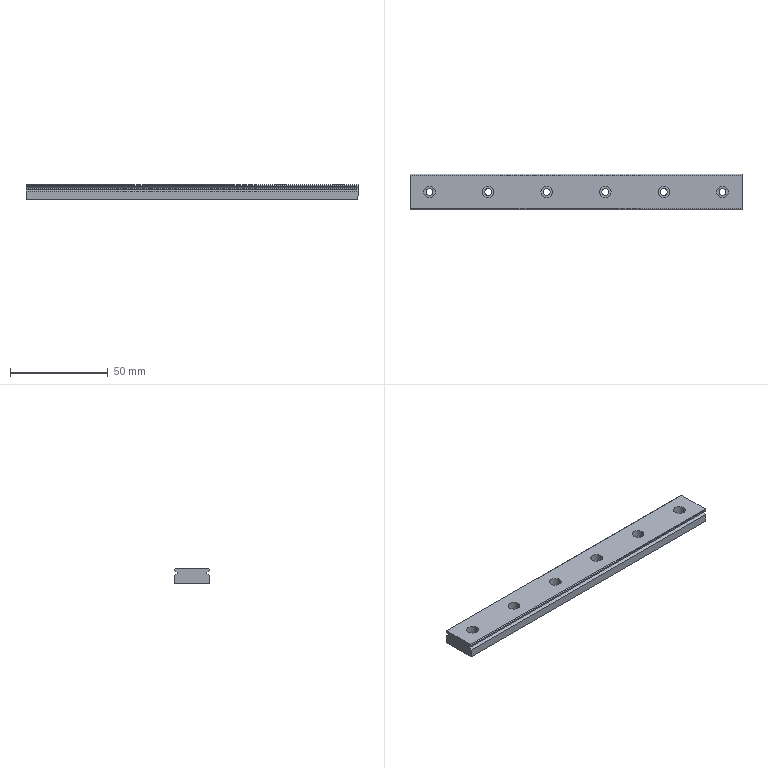Part | SolidWorks | features BaseBody 1 | 1 solid | 46 faces | box 170 x 18 x 7.5 mm | volume 21263 mm3 | cylinder 24 | plane 22 | commonest cylinder face diameters 3.5 x12 6 x12
STEP:
#1=CARTESIAN_POINT('',(-91.75,0.,0.));
#2=VERTEX_POINT('',#1);
#3=CARTESIAN_POINT('',(-88.25,0.,0.));
#4=VERTEX_POINT('',#3);
#5=CARTESIAN_POINT('',(-90.,0.,0.));
#6=DIRECTION('',(0.,0.,1.));
#7=DIRECTION('',(1.,0.,0.));
#8=AXIS2_PLACEMENT_3D('',#5,#6,#7);
#9=CIRCLE('',#8,1.75);
#10=EDGE_CURVE('',#2,#4,#9,.T.);
#11=ORIENTED_EDGE('',*,*,#10,.F.);
#12=CARTESIAN_POINT('',(-91.75,0.,3.));
#13=VERTEX_POINT('',#12);
#14=CARTESIAN_POINT('',(-91.75,0.,-1.163));
#15=DIRECTION('',(0.,0.,1.));
#16=VECTOR('',#15,1000.);
#17=LINE('',#14,#16);
#18=EDGE_CURVE('',#2,#13,#17,.T.);
#19=ORIENTED_EDGE('',*,*,#18,.T.);
#20=CARTESIAN_POINT('',(-88.25,0.,3.));
#21=VERTEX_POINT('',#20);
#22=CARTESIAN_POINT('',(-90.,0.,3.));
#23=DIRECTION('',(0.,0.,-1.));
#24=DIRECTION('',(1.,0.,0.));
#25=AXIS2_PLACEMENT_3D('',#22,#23,#24);
#26=CIRCLE('',#25,1.75);
#27=EDGE_CURVE('',#21,#13,#26,.T.);
#28=ORIENTED_EDGE('',*,*,#27,.F.);
#29=CARTESIAN_POINT('',(-88.25,0.,-1.163));
#30=DIRECTION('',(0.,0.,1.));
#31=VECTOR('',#30,1000.);
#32=LINE('',#29,#31);
#33=EDGE_CURVE('',#4,#21,#32,.T.);
#34=ORIENTED_EDGE('',*,*,#33,.F.);
#35=EDGE_LOOP('',(#11,#19,#28,#34));
#36=FACE_OUTER_BOUND('',#35,.T.);
#37=CARTESIAN_POINT('',(-90.,0.,-1.163));
#38=DIRECTION('',(0.,0.,1.));
#39=DIRECTION('',(1.,0.,0.));
#40=AXIS2_PLACEMENT_3D('',#37,#38,#39);
#41=CYLINDRICAL_SURFACE('',#40,1.75);
#42=ADVANCED_FACE('',(#36),#41,.F.);
#43=CARTESIAN_POINT('',(-61.75,0.,0.));
#44=VERTEX_POINT('',#43);
#45=CARTESIAN_POINT('',(-58.25,0.,0.));
#46=VERTEX_POINT('',#45);
#47=CARTESIAN_POINT('',(-60.,0.,0.));
#48=DIRECTION('',(0.,0.,1.));
#49=DIRECTION('',(1.,0.,0.));
#50=AXIS2_PLACEMENT_3D('',#47,#48,#49);
#51=CIRCLE('',#50,1.75);
#52=EDGE_CURVE('',#44,#46,#51,.T.);
#53=ORIENTED_EDGE('',*,*,#52,.F.);
#54=CARTESIAN_POINT('',(-61.75,0.,3.));
#55=VERTEX_POINT('',#54);
#56=CARTESIAN_POINT('',(-61.75,0.,-1.163));
#57=DIRECTION('',(0.,0.,1.));
#58=VECTOR('',#57,1000.);
#59=LINE('',#56,#58);
#60=EDGE_CURVE('',#44,#55,#59,.T.);
#61=ORIENTED_EDGE('',*,*,#60,.T.);
#62=CARTESIAN_POINT('',(-58.25,0.,3.));
#63=VERTEX_POINT('',#62);
#64=CARTESIAN_POINT('',(-60.,0.,3.));
#65=DIRECTION('',(0.,0.,-1.));
#66=DIRECTION('',(1.,0.,0.));
#67=AXIS2_PLACEMENT_3D('',#64,#65,#66);
#68=CIRCLE('',#67,1.75);
#69=EDGE_CURVE('',#63,#55,#68,.T.);
#70=ORIENTED_EDGE('',*,*,#69,.F.);
#71=CARTESIAN_POINT('',(-58.25,0.,-1.163));
#72=DIRECTION('',(0.,0.,1.));
#73=VECTOR('',#72,1000.);
#74=LINE('',#71,#73);
#75=EDGE_CURVE('',#46,#63,#74,.T.);
#76=ORIENTED_EDGE('',*,*,#75,.F.);
#77=EDGE_LOOP('',(#53,#61,#70,#76));
#78=FACE_OUTER_BOUND('',#77,.T.);
#79=CARTESIAN_POINT('',(-60.,0.,-1.163));
#80=DIRECTION('',(0.,0.,1.));
#81=DIRECTION('',(1.,0.,0.));
#82=AXIS2_PLACEMENT_3D('',#79,#80,#81);
#83=CYLINDRICAL_SURFACE('',#82,1.75);
#84=ADVANCED_FACE('',(#78),#83,.F.);
#85=CARTESIAN_POINT('',(-31.75,0.,0.));
#86=VERTEX_POINT('',#85);
#87=CARTESIAN_POINT('',(-28.25,0.,0.));
#88=VERTEX_POINT('',#87);
#89=CARTESIAN_POINT('',(-30.,0.,0.));
#90=DIRECTION('',(0.,0.,1.));
#91=DIRECTION('',(1.,0.,0.));
#92=AXIS2_PLACEMENT_3D('',#89,#90,#91);
#93=CIRCLE('',#92,1.75);
#94=EDGE_CURVE('',#86,#88,#93,.T.);
#95=ORIENTED_EDGE('',*,*,#94,.F.);
#96=CARTESIAN_POINT('',(-31.75,0.,3.));
#97=VERTEX_POINT('',#96);
#98=CARTESIAN_POINT('',(-31.75,0.,-1.163));
#99=DIRECTION('',(0.,0.,1.));
#100=VECTOR('',#99,1000.);
#101=LINE('',#98,#100);
#102=EDGE_CURVE('',#86,#97,#101,.T.);
#103=ORIENTED_EDGE('',*,*,#102,.T.);
#104=CARTESIAN_POINT('',(-28.25,0.,3.));
#105=VERTEX_POINT('',#104);
#106=CARTESIAN_POINT('',(-30.,0.,3.));
#107=DIRECTION('',(0.,0.,-1.));
#108=DIRECTION('',(1.,0.,0.));
#109=AXIS2_PLACEMENT_3D('',#106,#107,#108);
#110=CIRCLE('',#109,1.75);
#111=EDGE_CURVE('',#105,#97,#110,.T.);
#112=ORIENTED_EDGE('',*,*,#111,.F.);
#113=CARTESIAN_POINT('',(-28.25,0.,-1.163));
#114=DIRECTION('',(0.,0.,1.));
#115=VECTOR('',#114,1000.);
#116=LINE('',#113,#115);
#117=EDGE_CURVE('',#88,#105,#116,.T.);
#118=ORIENTED_EDGE('',*,*,#117,.F.);
#119=EDGE_LOOP('',(#95,#103,#112,#118));
#120=FACE_OUTER_BOUND('',#119,.T.);
#121=CARTESIAN_POINT('',(-30.,0.,-1.163));
#122=DIRECTION('',(0.,0.,1.));
#123=DIRECTION('',(1.,0.,0.));
#124=AXIS2_PLACEMENT_3D('',#121,#122,#123);
#125=CYLINDRICAL_SURFACE('',#124,1.75);
#126=ADVANCED_FACE('',(#120),#125,.F.);
#127=CARTESIAN_POINT('',(58.25,0.,0.));
#128=VERTEX_POINT('',#127);
#129=CARTESIAN_POINT('',(61.75,0.,0.));
#130=VERTEX_POINT('',#129);
#131=CARTESIAN_POINT('',(60.,0.,0.));
#132=DIRECTION('',(0.,0.,1.));
#133=DIRECTION('',(1.,0.,0.));
#134=AXIS2_PLACEMENT_3D('',#131,#132,#133);
#135=CIRCLE('',#134,1.75);
#136=EDGE_CURVE('',#128,#130,#135,.T.);
#137=ORIENTED_EDGE('',*,*,#136,.F.);
#138=CARTESIAN_POINT('',(58.25,0.,3.));
#139=VERTEX_POINT('',#138);
#140=CARTESIAN_POINT('',(58.25,0.,1.5));
#141=DIRECTION('',(0.,0.,1.));
#142=VECTOR('',#141,1000.);
#143=LINE('',#140,#142);
#144=EDGE_CURVE('',#128,#139,#143,.T.);
#145=ORIENTED_EDGE('',*,*,#144,.T.);
#146=CARTESIAN_POINT('',(61.75,0.,3.));
#147=VERTEX_POINT('',#146);
#148=CARTESIAN_POINT('',(60.,0.,3.));
#149=DIRECTION('',(0.,0.,-1.));
#150=DIRECTION('',(1.,0.,0.));
#151=AXIS2_PLACEMENT_3D('',#148,#149,#150);
#152=CIRCLE('',#151,1.75);
#153=EDGE_CURVE('',#147,#139,#152,.T.);
#154=ORIENTED_EDGE('',*,*,#153,.F.);
#155=CARTESIAN_POINT('',(61.75,0.,1.5));
#156=DIRECTION('',(0.,0.,1.));
#157=VECTOR('',#156,1000.);
#158=LINE('',#155,#157);
#159=EDGE_CURVE('',#130,#147,#158,.T.);
#160=ORIENTED_EDGE('',*,*,#159,.F.);
#161=EDGE_LOOP('',(#137,#145,#154,#160));
#162=FACE_OUTER_BOUND('',#161,.T.);
#163=CARTESIAN_POINT('',(60.,0.,1.5));
#164=DIRECTION('',(0.,0.,1.));
#165=DIRECTION('',(1.,0.,0.));
#166=AXIS2_PLACEMENT_3D('',#163,#164,#165);
#167=CYLINDRICAL_SURFACE('',#166,1.75);
#168=ADVANCED_FACE('',(#162),#167,.F.);
#169=CARTESIAN_POINT('',(-1.75,0.,0.));
#170=VERTEX_POINT('',#169);
#171=CARTESIAN_POINT('',(1.75,0.,0.));
#172=VERTEX_POINT('',#171);
#173=CARTESIAN_POINT('',(0.,0.,0.));
#174=DIRECTION('',(0.,0.,1.));
#175=DIRECTION('',(1.,0.,0.));
#176=AXIS2_PLACEMENT_3D('',#173,#174,#175);
#177=CIRCLE('',#176,1.75);
#178=EDGE_CURVE('',#170,#172,#177,.T.);
#179=ORIENTED_EDGE('',*,*,#178,.F.);
#180=CARTESIAN_POINT('',(-1.75,0.,3.));
#181=VERTEX_POINT('',#180);
#182=CARTESIAN_POINT('',(-1.75,0.,1.5));
#183=DIRECTION('',(0.,0.,1.));
#184=VECTOR('',#183,1000.);
#185=LINE('',#182,#184);
#186=EDGE_CURVE('',#170,#181,#185,.T.);
#187=ORIENTED_EDGE('',*,*,#186,.T.);
#188=CARTESIAN_POINT('',(1.75,0.,3.));
#189=VERTEX_POINT('',#188);
#190=CARTESIAN_POINT('',(0.,0.,3.));
#191=DIRECTION('',(0.,0.,-1.));
#192=DIRECTION('',(1.,0.,0.));
#193=AXIS2_PLACEMENT_3D('',#190,#191,#192);
#194=CIRCLE('',#193,1.75);
#195=EDGE_CURVE('',#189,#181,#194,.T.);
#196=ORIENTED_EDGE('',*,*,#195,.F.);
#197=CARTESIAN_POINT('',(1.75,0.,1.5));
#198=DIRECTION('',(0.,0.,1.));
#199=VECTOR('',#198,1000.);
#200=LINE('',#197,#199);
#201=EDGE_CURVE('',#172,#189,#200,.T.);
#202=ORIENTED_EDGE('',*,*,#201,.F.);
#203=EDGE_LOOP('',(#179,#187,#196,#202));
#204=FACE_OUTER_BOUND('',#203,.T.);
#205=CARTESIAN_POINT('',(0.,0.,1.5));
#206=DIRECTION('',(0.,0.,1.));
#207=DIRECTION('',(1.,0.,0.));
#208=AXIS2_PLACEMENT_3D('',#205,#206,#207);
#209=CYLINDRICAL_SURFACE('',#208,1.75);
#210=ADVANCED_FACE('',(#204),#209,.F.);
#211=CARTESIAN_POINT('',(28.25,0.,0.));
#212=VERTEX_POINT('',#211);
#213=CARTESIAN_POINT('',(31.75,0.,0.));
#214=VERTEX_POINT('',#213);
#215=CARTESIAN_POINT('',(30.,0.,0.));
#216=DIRECTION('',(0.,0.,1.));
#217=DIRECTION('',(1.,0.,0.));
#218=AXIS2_PLACEMENT_3D('',#215,#216,#217);
#219=CIRCLE('',#218,1.75);
#220=EDGE_CURVE('',#212,#214,#219,.T.);
#221=ORIENTED_EDGE('',*,*,#220,.F.);
#222=CARTESIAN_POINT('',(28.25,0.,3.));
#223=VERTEX_POINT('',#222);
#224=CARTESIAN_POINT('',(28.25,0.,1.5));
#225=DIRECTION('',(0.,0.,1.));
#226=VECTOR('',#225,1000.);
#227=LINE('',#224,#226);
#228=EDGE_CURVE('',#212,#223,#227,.T.);
#229=ORIENTED_EDGE('',*,*,#228,.T.);
#230=CARTESIAN_POINT('',(31.75,0.,3.));
#231=VERTEX_POINT('',#230);
#232=CARTESIAN_POINT('',(30.,0.,3.));
#233=DIRECTION('',(0.,0.,-1.));
#234=DIRECTION('',(1.,0.,0.));
#235=AXIS2_PLACEMENT_3D('',#232,#233,#234);
#236=CIRCLE('',#235,1.75);
#237=EDGE_CURVE('',#231,#223,#236,.T.);
#238=ORIENTED_EDGE('',*,*,#237,.F.);
#239=CARTESIAN_POINT('',(31.75,0.,1.5));
#240=DIRECTION('',(0.,0.,1.));
#241=VECTOR('',#240,1000.);
#242=LINE('',#239,#241);
#243=EDGE_CURVE('',#214,#231,#242,.T.);
#244=ORIENTED_EDGE('',*,*,#243,.F.);
#245=EDGE_LOOP('',(#221,#229,#238,#244));
#246=FACE_OUTER_BOUND('',#245,.T.);
#247=CARTESIAN_POINT('',(30.,0.,1.5));
#248=DIRECTION('',(0.,0.,1.));
#249=DIRECTION('',(1.,0.,0.));
#250=AXIS2_PLACEMENT_3D('',#247,#248,#249);
#251=CYLINDRICAL_SURFACE('',#250,1.75);
#252=ADVANCED_FACE('',(#246),#251,.F.);
#253=CARTESIAN_POINT('',(-93.,0.,3.));
#254=VERTEX_POINT('',#253);
#255=CARTESIAN_POINT('',(-87.,0.,3.));
#256=VERTEX_POINT('',#255);
#257=CARTESIAN_POINT('',(-90.,0.,3.));
#258=DIRECTION('',(0.,0.,1.));
#259=DIRECTION('',(1.,0.,0.));
#260=AXIS2_PLACEMENT_3D('',#257,#258,#259);
#261=CIRCLE('',#260,3.);
#262=EDGE_CURVE('',#254,#256,#261,.T.);
#263=ORIENTED_EDGE('',*,*,#262,.F.);
#264=CARTESIAN_POINT('',(-93.,0.,7.5));
#265=VERTEX_POINT('',#264);
#266=CARTESIAN_POINT('',(-93.,0.,-1.163));
#267=DIRECTION('',(0.,0.,1.));
#268=VECTOR('',#267,1000.);
#269=LINE('',#266,#268);
#270=EDGE_CURVE('',#254,#265,#269,.T.);
#271=ORIENTED_EDGE('',*,*,#270,.T.);
#272=CARTESIAN_POINT('',(-87.,0.,7.5));
#273=VERTEX_POINT('',#272);
#274=CARTESIAN_POINT('',(-90.,0.,7.5));
#275=DIRECTION('',(0.,0.,-1.));
#276=DIRECTION('',(1.,0.,0.));
#277=AXIS2_PLACEMENT_3D('',#274,#275,#276);
#278=CIRCLE('',#277,3.);
#279=EDGE_CURVE('',#273,#265,#278,.T.);
#280=ORIENTED_EDGE('',*,*,#279,.F.);
#281=CARTESIAN_POINT('',(-87.,0.,-1.163));
#282=DIRECTION('',(0.,0.,1.));
#283=VECTOR('',#282,1000.);
#284=LINE('',#281,#283);
#285=EDGE_CURVE('',#256,#273,#284,.T.);
#286=ORIENTED_EDGE('',*,*,#285,.F.);
#287=EDGE_LOOP('',(#263,#271,#280,#286));
#288=FACE_OUTER_BOUND('',#287,.T.);
#289=CARTESIAN_POINT('',(-90.,0.,-1.163));
#290=DIRECTION('',(0.,0.,1.));
#291=DIRECTION('',(1.,0.,0.));
#292=AXIS2_PLACEMENT_3D('',#289,#290,#291);
#293=CYLINDRICAL_SURFACE('',#292,3.);
#294=ADVANCED_FACE('',(#288),#293,.F.);
#295=CARTESIAN_POINT('',(-63.,0.,3.));
#296=VERTEX_POINT('',#295);
#297=CARTESIAN_POINT('',(-57.,0.,3.));
#298=VERTEX_POINT('',#297);
#299=CARTESIAN_POINT('',(-60.,0.,3.));
#300=DIRECTION('',(0.,0.,1.));
#301=DIRECTION('',(1.,0.,0.));
#302=AXIS2_PLACEMENT_3D('',#299,#300,#301);
#303=CIRCLE('',#302,3.);
#304=EDGE_CURVE('',#296,#298,#303,.T.);
#305=ORIENTED_EDGE('',*,*,#304,.F.);
#306=CARTESIAN_POINT('',(-63.,0.,7.5));
#307=VERTEX_POINT('',#306);
#308=CARTESIAN_POINT('',(-63.,0.,-1.163));
#309=DIRECTION('',(0.,0.,1.));
#310=VECTOR('',#309,1000.);
#311=LINE('',#308,#310);
#312=EDGE_CURVE('',#296,#307,#311,.T.);
#313=ORIENTED_EDGE('',*,*,#312,.T.);
#314=CARTESIAN_POINT('',(-57.,0.,7.5));
#315=VERTEX_POINT('',#314);
#316=CARTESIAN_POINT('',(-60.,0.,7.5));
#317=DIRECTION('',(0.,0.,-1.));
#318=DIRECTION('',(1.,0.,0.));
#319=AXIS2_PLACEMENT_3D('',#316,#317,#318);
#320=CIRCLE('',#319,3.);
#321=EDGE_CURVE('',#315,#307,#320,.T.);
#322=ORIENTED_EDGE('',*,*,#321,.F.);
#323=CARTESIAN_POINT('',(-57.,0.,-1.163));
#324=DIRECTION('',(0.,0.,1.));
#325=VECTOR('',#324,1000.);
#326=LINE('',#323,#325);
#327=EDGE_CURVE('',#298,#315,#326,.T.);
#328=ORIENTED_EDGE('',*,*,#327,.F.);
#329=EDGE_LOOP('',(#305,#313,#322,#328));
#330=FACE_OUTER_BOUND('',#329,.T.);
#331=CARTESIAN_POINT('',(-60.,0.,-1.163));
#332=DIRECTION('',(0.,0.,1.));
#333=DIRECTION('',(1.,0.,0.));
#334=AXIS2_PLACEMENT_3D('',#331,#332,#333);
#335=CYLINDRICAL_SURFACE('',#334,3.);
#336=ADVANCED_FACE('',(#330),#335,.F.);
#337=CARTESIAN_POINT('',(-33.,0.,3.));
#338=VERTEX_POINT('',#337);
#339=CARTESIAN_POINT('',(-27.,0.,3.));
#340=VERTEX_POINT('',#339);
#341=CARTESIAN_POINT('',(-30.,0.,3.));
#342=DIRECTION('',(0.,0.,1.));
#343=DIRECTION('',(1.,0.,0.));
#344=AXIS2_PLACEMENT_3D('',#341,#342,#343);
#345=CIRCLE('',#344,3.);
#346=EDGE_CURVE('',#338,#340,#345,.T.);
#347=ORIENTED_EDGE('',*,*,#346,.F.);
#348=CARTESIAN_POINT('',(-33.,0.,7.5));
#349=VERTEX_POINT('',#348);
#350=CARTESIAN_POINT('',(-33.,0.,-1.163));
#351=DIRECTION('',(0.,0.,1.));
#352=VECTOR('',#351,1000.);
#353=LINE('',#350,#352);
#354=EDGE_CURVE('',#338,#349,#353,.T.);
#355=ORIENTED_EDGE('',*,*,#354,.T.);
#356=CARTESIAN_POINT('',(-27.,0.,7.5));
#357=VERTEX_POINT('',#356);
#358=CARTESIAN_POINT('',(-30.,0.,7.5));
#359=DIRECTION('',(0.,0.,-1.));
#360=DIRECTION('',(1.,0.,0.));
#361=AXIS2_PLACEMENT_3D('',#358,#359,#360);
#362=CIRCLE('',#361,3.);
#363=EDGE_CURVE('',#357,#349,#362,.T.);
#364=ORIENTED_EDGE('',*,*,#363,.F.);
#365=CARTESIAN_POINT('',(-27.,0.,-1.163));
#366=DIRECTION('',(0.,0.,1.));
#367=VECTOR('',#366,1000.);
#368=LINE('',#365,#367);
#369=EDGE_CURVE('',#340,#357,#368,.T.);
#370=ORIENTED_EDGE('',*,*,#369,.F.);
#371=EDGE_LOOP('',(#347,#355,#364,#370));
#372=FACE_OUTER_BOUND('',#371,.T.);
#373=CARTESIAN_POINT('',(-30.,0.,-1.163));
#374=DIRECTION('',(0.,0.,1.));
#375=DIRECTION('',(1.,0.,0.));
#376=AXIS2_PLACEMENT_3D('',#373,#374,#375);
#377=CYLINDRICAL_SURFACE('',#376,3.);
#378=ADVANCED_FACE('',(#372),#377,.F.);
#379=CARTESIAN_POINT('',(63.,0.,7.5));
#380=VERTEX_POINT('',#379);
#381=CARTESIAN_POINT('',(57.,0.,7.5));
#382=VERTEX_POINT('',#381);
#383=CARTESIAN_POINT('',(60.,0.,7.5));
#384=DIRECTION('',(0.,0.,-1.));
#385=DIRECTION('',(-1.,0.,0.));
#386=AXIS2_PLACEMENT_3D('',#383,#384,#385);
#387=CIRCLE('',#386,3.);
#388=EDGE_CURVE('',#380,#382,#387,.T.);
#389=ORIENTED_EDGE('',*,*,#388,.F.);
#390=CARTESIAN_POINT('',(63.,0.,3.));
#391=VERTEX_POINT('',#390);
#392=CARTESIAN_POINT('',(63.,0.,5.25));
#393=DIRECTION('',(0.,0.,-1.));
#394=VECTOR('',#393,1000.);
#395=LINE('',#392,#394);
#396=EDGE_CURVE('',#380,#391,#395,.T.);
#397=ORIENTED_EDGE('',*,*,#396,.T.);
#398=CARTESIAN_POINT('',(57.,0.,3.));
#399=VERTEX_POINT('',#398);
#400=CARTESIAN_POINT('',(60.,0.,3.));
#401=DIRECTION('',(0.,0.,-1.));
#402=DIRECTION('',(-1.,0.,0.));
#403=AXIS2_PLACEMENT_3D('',#400,#401,#402);
#404=CIRCLE('',#403,3.);
#405=EDGE_CURVE('',#391,#399,#404,.T.);
#406=ORIENTED_EDGE('',*,*,#405,.T.);
#407=CARTESIAN_POINT('',(57.,0.,5.25));
#408=DIRECTION('',(0.,0.,-1.));
#409=VECTOR('',#408,1000.);
#410=LINE('',#407,#409);
#411=EDGE_CURVE('',#382,#399,#410,.T.);
#412=ORIENTED_EDGE('',*,*,#411,.F.);
#413=EDGE_LOOP('',(#389,#397,#406,#412));
#414=FACE_OUTER_BOUND('',#413,.T.);
#415=CARTESIAN_POINT('',(60.,0.,5.25));
#416=DIRECTION('',(0.,0.,-1.));
#417=DIRECTION('',(-1.,0.,0.));
#418=AXIS2_PLACEMENT_3D('',#415,#416,#417);
#419=CYLINDRICAL_SURFACE('',#418,3.);
#420=ADVANCED_FACE('',(#414),#419,.F.);
#421=CARTESIAN_POINT('',(3.,0.,7.5));
#422=VERTEX_POINT('',#421);
#423=CARTESIAN_POINT('',(-3.,0.,7.5));
#424=VERTEX_POINT('',#423);
#425=CARTESIAN_POINT('',(0.,0.,7.5));
#426=DIRECTION('',(0.,0.,-1.));
#427=DIRECTION('',(-1.,0.,0.));
#428=AXIS2_PLACEMENT_3D('',#425,#426,#427);
#429=CIRCLE('',#428,3.);
#430=EDGE_CURVE('',#422,#424,#429,.T.);
#431=ORIENTED_EDGE('',*,*,#430,.F.);
#432=CARTESIAN_POINT('',(3.,0.,3.));
#433=VERTEX_POINT('',#432);
#434=CARTESIAN_POINT('',(3.,0.,5.25));
#435=DIRECTION('',(0.,0.,-1.));
#436=VECTOR('',#435,1000.);
#437=LINE('',#434,#436);
#438=EDGE_CURVE('',#422,#433,#437,.T.);
#439=ORIENTED_EDGE('',*,*,#438,.T.);
#440=CARTESIAN_POINT('',(-3.,0.,3.));
#441=VERTEX_POINT('',#440);
#442=CARTESIAN_POINT('',(0.,0.,3.));
#443=DIRECTION('',(0.,0.,-1.));
#444=DIRECTION('',(-1.,0.,0.));
#445=AXIS2_PLACEMENT_3D('',#442,#443,#444);
#446=CIRCLE('',#445,3.);
#447=EDGE_CURVE('',#433,#441,#446,.T.);
#448=ORIENTED_EDGE('',*,*,#447,.T.);
#449=CARTESIAN_POINT('',(-3.,0.,5.25));
#450=DIRECTION('',(0.,0.,-1.));
#451=VECTOR('',#450,1000.);
#452=LINE('',#449,#451);
#453=EDGE_CURVE('',#424,#441,#452,.T.);
#454=ORIENTED_EDGE('',*,*,#453,.F.);
#455=EDGE_LOOP('',(#431,#439,#448,#454));
#456=FACE_OUTER_BOUND('',#455,.T.);
#457=CARTESIAN_POINT('',(0.,0.,5.25));
#458=DIRECTION('',(0.,0.,-1.));
#459=DIRECTION('',(-1.,0.,0.));
#460=AXIS2_PLACEMENT_3D('',#457,#458,#459);
#461=CYLINDRICAL_SURFACE('',#460,3.);
#462=ADVANCED_FACE('',(#456),#461,.F.);
#463=CARTESIAN_POINT('',(33.,0.,7.5));
#464=VERTEX_POINT('',#463);
#465=CARTESIAN_POINT('',(27.,0.,7.5));
#466=VERTEX_POINT('',#465);
#467=CARTESIAN_POINT('',(30.,0.,7.5));
#468=DIRECTION('',(0.,0.,-1.));
#469=DIRECTION('',(-1.,0.,0.));
#470=AXIS2_PLACEMENT_3D('',#467,#468,#469);
#471=CIRCLE('',#470,3.);
#472=EDGE_CURVE('',#464,#466,#471,.T.);
#473=ORIENTED_EDGE('',*,*,#472,.F.);
#474=CARTESIAN_POINT('',(33.,0.,3.));
#475=VERTEX_POINT('',#474);
#476=CARTESIAN_POINT('',(33.,0.,5.25));
#477=DIRECTION('',(0.,0.,-1.));
#478=VECTOR('',#477,1000.);
#479=LINE('',#476,#478);
#480=EDGE_CURVE('',#464,#475,#479,.T.);
#481=ORIENTED_EDGE('',*,*,#480,.T.);
#482=CARTESIAN_POINT('',(27.,0.,3.));
#483=VERTEX_POINT('',#482);
#484=CARTESIAN_POINT('',(30.,0.,3.));
#485=DIRECTION('',(0.,0.,-1.));
#486=DIRECTION('',(-1.,0.,0.));
#487=AXIS2_PLACEMENT_3D('',#484,#485,#486);
#488=CIRCLE('',#487,3.);
#489=EDGE_CURVE('',#475,#483,#488,.T.);
#490=ORIENTED_EDGE('',*,*,#489,.T.);
#491=CARTESIAN_POINT('',(27.,0.,5.25));
#492=DIRECTION('',(0.,0.,-1.));
#493=VECTOR('',#492,1000.);
#494=LINE('',#491,#493);
#495=EDGE_CURVE('',#466,#483,#494,.T.);
#496=ORIENTED_EDGE('',*,*,#495,.F.);
#497=EDGE_LOOP('',(#473,#481,#490,#496));
#498=FACE_OUTER_BOUND('',#497,.T.);
#499=CARTESIAN_POINT('',(30.,0.,5.25));
#500=DIRECTION('',(0.,0.,-1.));
#501=DIRECTION('',(-1.,0.,0.));
#502=AXIS2_PLACEMENT_3D('',#499,#500,#501);
#503=CYLINDRICAL_SURFACE('',#502,3.);
#504=ADVANCED_FACE('',(#498),#503,.F.);
#505=CARTESIAN_POINT('',(-90.,0.,0.));
#506=DIRECTION('',(0.,0.,1.));
#507=DIRECTION('',(1.,0.,0.));
#508=AXIS2_PLACEMENT_3D('',#505,#506,#507);
#509=CIRCLE('',#508,1.75);
#510=EDGE_CURVE('',#4,#2,#509,.T.);
#511=ORIENTED_EDGE('',*,*,#510,.T.);
#512=ORIENTED_EDGE('',*,*,#10,.T.);
#513=EDGE_LOOP('',(#511,#512));
#514=FACE_BOUND('',#513,.T.);
#515=CARTESIAN_POINT('',(-60.,0.,0.));
#516=DIRECTION('',(0.,0.,1.));
#517=DIRECTION('',(1.,0.,0.));
#518=AXIS2_PLACEMENT_3D('',#515,#516,#517);
#519=CIRCLE('',#518,1.75);
#520=EDGE_CURVE('',#46,#44,#519,.T.);
#521=ORIENTED_EDGE('',*,*,#520,.T.);
#522=ORIENTED_EDGE('',*,*,#52,.T.);
#523=EDGE_LOOP('',(#521,#522));
#524=FACE_BOUND('',#523,.T.);
#525=CARTESIAN_POINT('',(-30.,0.,0.));
#526=DIRECTION('',(0.,0.,1.));
#527=DIRECTION('',(1.,0.,0.));
#528=AXIS2_PLACEMENT_3D('',#525,#526,#527);
#529=CIRCLE('',#528,1.75);
#530=EDGE_CURVE('',#88,#86,#529,.T.);
#531=ORIENTED_EDGE('',*,*,#530,.T.);
#532=ORIENTED_EDGE('',*,*,#94,.T.);
#533=EDGE_LOOP('',(#531,#532));
#534=FACE_BOUND('',#533,.T.);
#535=CARTESIAN_POINT('',(60.,0.,0.));
#536=DIRECTION('',(0.,0.,1.));
#537=DIRECTION('',(1.,0.,0.));
#538=AXIS2_PLACEMENT_3D('',#535,#536,#537);
#539=CIRCLE('',#538,1.75);
#540=EDGE_CURVE('',#130,#128,#539,.T.);
#541=ORIENTED_EDGE('',*,*,#540,.T.);
#542=ORIENTED_EDGE('',*,*,#136,.T.);
#543=EDGE_LOOP('',(#541,#542));
#544=FACE_BOUND('',#543,.T.);
#545=CARTESIAN_POINT('',(0.,0.,0.));
#546=DIRECTION('',(0.,0.,1.));
#547=DIRECTION('',(1.,0.,0.));
#548=AXIS2_PLACEMENT_3D('',#545,#546,#547);
#549=CIRCLE('',#548,1.75);
#550=EDGE_CURVE('',#172,#170,#549,.T.);
#551=ORIENTED_EDGE('',*,*,#550,.T.);
#552=ORIENTED_EDGE('',*,*,#178,.T.);
#553=EDGE_LOOP('',(#551,#552));
#554=FACE_BOUND('',#553,.T.);
#555=CARTESIAN_POINT('',(30.,0.,0.));
#556=DIRECTION('',(0.,0.,1.));
#557=DIRECTION('',(1.,0.,0.));
#558=AXIS2_PLACEMENT_3D('',#555,#556,#557);
#559=CIRCLE('',#558,1.75);
#560=EDGE_CURVE('',#214,#212,#559,.T.);
#561=ORIENTED_EDGE('',*,*,#560,.T.);
#562=ORIENTED_EDGE('',*,*,#220,.T.);
#563=EDGE_LOOP('',(#561,#562));
#564=FACE_BOUND('',#563,.T.);
#565=CARTESIAN_POINT('',(-100.,-9.,0.));
#566=VERTEX_POINT('',#565);
#567=CARTESIAN_POINT('',(-100.,9.,0.));
#568=VERTEX_POINT('',#567);
#569=CARTESIAN_POINT('',(-100.,0.,0.));
#570=DIRECTION('',(0.,1.,0.));
#571=VECTOR('',#570,1000.);
#572=LINE('',#569,#571);
#573=EDGE_CURVE('',#566,#568,#572,.T.);
#574=ORIENTED_EDGE('',*,*,#573,.T.);
#575=CARTESIAN_POINT('',(70.,9.,0.));
#576=VERTEX_POINT('',#575);
#577=CARTESIAN_POINT('',(-10.,9.,0.));
#578=DIRECTION('',(1.,0.,0.));
#579=VECTOR('',#578,1000.);
#580=LINE('',#577,#579);
#581=EDGE_CURVE('',#568,#576,#580,.T.);
#582=ORIENTED_EDGE('',*,*,#581,.T.);
#583=CARTESIAN_POINT('',(70.,-9.,0.));
#584=VERTEX_POINT('',#583);
#585=CARTESIAN_POINT('',(70.,0.,0.));
#586=DIRECTION('',(0.,-1.,0.));
#587=VECTOR('',#586,1000.);
#588=LINE('',#585,#587);
#589=EDGE_CURVE('',#576,#584,#588,.T.);
#590=ORIENTED_EDGE('',*,*,#589,.T.);
#591=CARTESIAN_POINT('',(-10.,-9.,0.));
#592=DIRECTION('',(-1.,0.,0.));
#593=VECTOR('',#592,1000.);
#594=LINE('',#591,#593);
#595=EDGE_CURVE('',#584,#566,#594,.T.);
#596=ORIENTED_EDGE('',*,*,#595,.T.);
#597=EDGE_LOOP('',(#574,#582,#590,#596));
#598=FACE_OUTER_BOUND('',#597,.T.);
#599=CARTESIAN_POINT('',(-10.,0.,0.));
#600=DIRECTION('',(0.,0.,-1.));
#601=DIRECTION('',(-1.,0.,0.));
#602=AXIS2_PLACEMENT_3D('',#599,#600,#601);
#603=PLANE('',#602);
#604=ADVANCED_FACE('',(#514,#524,#534,#544,#554,#564,#598),#603,.T.);
#605=ORIENTED_EDGE('',*,*,#18,.F.);
#606=ORIENTED_EDGE('',*,*,#510,.F.);
#607=ORIENTED_EDGE('',*,*,#33,.T.);
#608=CARTESIAN_POINT('',(-90.,0.,3.));
#609=DIRECTION('',(0.,0.,-1.));
#610=DIRECTION('',(1.,0.,0.));
#611=AXIS2_PLACEMENT_3D('',#608,#609,#610);
#612=CIRCLE('',#611,1.75);
#613=EDGE_CURVE('',#13,#21,#612,.T.);
#614=ORIENTED_EDGE('',*,*,#613,.F.);
#615=EDGE_LOOP('',(#605,#606,#607,#614));
#616=FACE_OUTER_BOUND('',#615,.T.);
#617=CARTESIAN_POINT('',(-90.,0.,-1.163));
#618=DIRECTION('',(0.,0.,1.));
#619=DIRECTION('',(1.,0.,0.));
#620=AXIS2_PLACEMENT_3D('',#617,#618,#619);
#621=CYLINDRICAL_SURFACE('',#620,1.75);
#622=ADVANCED_FACE('',(#616),#621,.F.);
#623=ORIENTED_EDGE('',*,*,#60,.F.);
#624=ORIENTED_EDGE('',*,*,#520,.F.);
#625=ORIENTED_EDGE('',*,*,#75,.T.);
#626=CARTESIAN_POINT('',(-60.,0.,3.));
#627=DIRECTION('',(0.,0.,-1.));
#628=DIRECTION('',(1.,0.,0.));
#629=AXIS2_PLACEMENT_3D('',#626,#627,#628);
#630=CIRCLE('',#629,1.75);
#631=EDGE_CURVE('',#55,#63,#630,.T.);
#632=ORIENTED_EDGE('',*,*,#631,.F.);
#633=EDGE_LOOP('',(#623,#624,#625,#632));
#634=FACE_OUTER_BOUND('',#633,.T.);
#635=CARTESIAN_POINT('',(-60.,0.,-1.163));
#636=DIRECTION('',(0.,0.,1.));
#637=DIRECTION('',(1.,0.,0.));
#638=AXIS2_PLACEMENT_3D('',#635,#636,#637);
#639=CYLINDRICAL_SURFACE('',#638,1.75);
#640=ADVANCED_FACE('',(#634),#639,.F.);
#641=ORIENTED_EDGE('',*,*,#102,.F.);
#642=ORIENTED_EDGE('',*,*,#530,.F.);
#643=ORIENTED_EDGE('',*,*,#117,.T.);
#644=CARTESIAN_POINT('',(-30.,0.,3.));
#645=DIRECTION('',(0.,0.,-1.));
#646=DIRECTION('',(1.,0.,0.));
#647=AXIS2_PLACEMENT_3D('',#644,#645,#646);
#648=CIRCLE('',#647,1.75);
#649=EDGE_CURVE('',#97,#105,#648,.T.);
#650=ORIENTED_EDGE('',*,*,#649,.F.);
#651=EDGE_LOOP('',(#641,#642,#643,#650));
#652=FACE_OUTER_BOUND('',#651,.T.);
#653=CARTESIAN_POINT('',(-30.,0.,-1.163));
#654=DIRECTION('',(0.,0.,1.));
#655=DIRECTION('',(1.,0.,0.));
#656=AXIS2_PLACEMENT_3D('',#653,#654,#655);
#657=CYLINDRICAL_SURFACE('',#656,1.75);
#658=ADVANCED_FACE('',(#652),#657,.F.);
#659=ORIENTED_EDGE('',*,*,#144,.F.);
#660=ORIENTED_EDGE('',*,*,#540,.F.);
#661=ORIENTED_EDGE('',*,*,#159,.T.);
#662=CARTESIAN_POINT('',(60.,0.,3.));
#663=DIRECTION('',(0.,0.,-1.));
#664=DIRECTION('',(1.,0.,0.));
#665=AXIS2_PLACEMENT_3D('',#662,#663,#664);
#666=CIRCLE('',#665,1.75);
#667=EDGE_CURVE('',#139,#147,#666,.T.);
#668=ORIENTED_EDGE('',*,*,#667,.F.);
#669=EDGE_LOOP('',(#659,#660,#661,#668));
#670=FACE_OUTER_BOUND('',#669,.T.);
#671=CARTESIAN_POINT('',(60.,0.,1.5));
#672=DIRECTION('',(0.,0.,1.));
#673=DIRECTION('',(1.,0.,0.));
#674=AXIS2_PLACEMENT_3D('',#671,#672,#673);
#675=CYLINDRICAL_SURFACE('',#674,1.75);
#676=ADVANCED_FACE('',(#670),#675,.F.);
#677=ORIENTED_EDGE('',*,*,#186,.F.);
#678=ORIENTED_EDGE('',*,*,#550,.F.);
#679=ORIENTED_EDGE('',*,*,#201,.T.);
#680=CARTESIAN_POINT('',(0.,0.,3.));
#681=DIRECTION('',(0.,0.,-1.));
#682=DIRECTION('',(1.,0.,0.));
#683=AXIS2_PLACEMENT_3D('',#680,#681,#682);
#684=CIRCLE('',#683,1.75);
#685=EDGE_CURVE('',#181,#189,#684,.T.);
#686=ORIENTED_EDGE('',*,*,#685,.F.);
#687=EDGE_LOOP('',(#677,#678,#679,#686));
#688=FACE_OUTER_BOUND('',#687,.T.);
#689=CARTESIAN_POINT('',(0.,0.,1.5));
#690=DIRECTION('',(0.,0.,1.));
#691=DIRECTION('',(1.,0.,0.));
#692=AXIS2_PLACEMENT_3D('',#689,#690,#691);
#693=CYLINDRICAL_SURFACE('',#692,1.75);
#694=ADVANCED_FACE('',(#688),#693,.F.);
#695=ORIENTED_EDGE('',*,*,#228,.F.);
#696=ORIENTED_EDGE('',*,*,#560,.F.);
#697=ORIENTED_EDGE('',*,*,#243,.T.);
#698=CARTESIAN_POINT('',(30.,0.,3.));
#699=DIRECTION('',(0.,0.,-1.));
#700=DIRECTION('',(1.,0.,0.));
#701=AXIS2_PLACEMENT_3D('',#698,#699,#700);
#702=CIRCLE('',#701,1.75);
#703=EDGE_CURVE('',#223,#231,#702,.T.);
#704=ORIENTED_EDGE('',*,*,#703,.F.);
#705=EDGE_LOOP('',(#695,#696,#697,#704));
#706=FACE_OUTER_BOUND('',#705,.T.);
#707=CARTESIAN_POINT('',(30.,0.,1.5));
#708=DIRECTION('',(0.,0.,1.));
#709=DIRECTION('',(1.,0.,0.));
#710=AXIS2_PLACEMENT_3D('',#707,#708,#709);
#711=CYLINDRICAL_SURFACE('',#710,1.75);
#712=ADVANCED_FACE('',(#706),#711,.F.);
#713=CARTESIAN_POINT('',(-100.,9.,4.2));
#714=VERTEX_POINT('',#713);
#715=CARTESIAN_POINT('',(-100.,9.,4.2));
#716=DIRECTION('',(0.,0.,1.));
#717=VECTOR('',#716,1000.);
#718=LINE('',#715,#717);
#719=EDGE_CURVE('',#568,#714,#718,.T.);
#720=ORIENTED_EDGE('',*,*,#719,.T.);
#721=CARTESIAN_POINT('',(70.,9.,4.2));
#722=VERTEX_POINT('',#721);
#723=CARTESIAN_POINT('',(-10.,9.,4.2));
#724=DIRECTION('',(1.,0.,0.));
#725=VECTOR('',#724,1000.);
#726=LINE('',#723,#725);
#727=EDGE_CURVE('',#714,#722,#726,.T.);
#728=ORIENTED_EDGE('',*,*,#727,.T.);
#729=CARTESIAN_POINT('',(70.,9.,4.2));
#730=DIRECTION('',(0.,0.,-1.));
#731=VECTOR('',#730,1000.);
#732=LINE('',#729,#731);
#733=EDGE_CURVE('',#722,#576,#732,.T.);
#734=ORIENTED_EDGE('',*,*,#733,.T.);
#735=ORIENTED_EDGE('',*,*,#581,.F.);
#736=EDGE_LOOP('',(#720,#728,#734,#735));
#737=FACE_OUTER_BOUND('',#736,.T.);
#738=CARTESIAN_POINT('',(-10.,9.,4.2));
#739=DIRECTION('',(0.,1.,0.));
#740=DIRECTION('',(0.,0.,1.));
#741=AXIS2_PLACEMENT_3D('',#738,#739,#740);
#742=PLANE('',#741);
#743=ADVANCED_FACE('',(#737),#742,.T.);
#744=ORIENTED_EDGE('',*,*,#719,.F.);
#745=ORIENTED_EDGE('',*,*,#573,.F.);
#746=CARTESIAN_POINT('',(-100.,-9.,4.2));
#747=VERTEX_POINT('',#746);
#748=CARTESIAN_POINT('',(-100.,-9.,0.));
#749=DIRECTION('',(0.,0.,1.));
#750=VECTOR('',#749,1000.);
#751=LINE('',#748,#750);
#752=EDGE_CURVE('',#566,#747,#751,.T.);
#753=ORIENTED_EDGE('',*,*,#752,.T.);
#754=CARTESIAN_POINT('',(-100.,-7.5,4.95));
#755=VERTEX_POINT('',#754);
#756=CARTESIAN_POINT('',(-100.,-9.,4.2));
#757=DIRECTION('',(0.,-0.8944,-0.4472));
#758=VECTOR('',#757,1000.);
#759=LINE('',#756,#758);
#760=EDGE_CURVE('',#755,#747,#759,.T.);
#761=ORIENTED_EDGE('',*,*,#760,.F.);
#762=CARTESIAN_POINT('',(-100.,-7.5,5.625));
#763=VERTEX_POINT('',#762);
#764=CARTESIAN_POINT('',(-100.,-7.5,4.95));
#765=DIRECTION('',(0.,0.,-1.));
#766=VECTOR('',#765,1000.);
#767=LINE('',#764,#766);
#768=EDGE_CURVE('',#763,#755,#767,.T.);
#769=ORIENTED_EDGE('',*,*,#768,.F.);
#770=CARTESIAN_POINT('',(-100.,-9.,6.375));
#771=VERTEX_POINT('',#770);
#772=CARTESIAN_POINT('',(-100.,-7.5,5.625));
#773=DIRECTION('',(0.,0.8944,-0.4472));
#774=VECTOR('',#773,1000.);
#775=LINE('',#772,#774);
#776=EDGE_CURVE('',#771,#763,#775,.T.);
#777=ORIENTED_EDGE('',*,*,#776,.F.);
#778=CARTESIAN_POINT('',(-100.,-9.,7.125));
#779=VERTEX_POINT('',#778);
#780=CARTESIAN_POINT('',(-100.,-9.,6.375));
#781=DIRECTION('',(0.,0.,-1.));
#782=VECTOR('',#781,1000.);
#783=LINE('',#780,#782);
#784=EDGE_CURVE('',#779,#771,#783,.T.);
#785=ORIENTED_EDGE('',*,*,#784,.F.);
#786=CARTESIAN_POINT('',(-100.,-8.625,7.5));
#787=VERTEX_POINT('',#786);
#788=CARTESIAN_POINT('',(-100.,-9.,7.125));
#789=DIRECTION('',(0.,-0.7071,-0.7071));
#790=VECTOR('',#789,1000.);
#791=LINE('',#788,#790);
#792=EDGE_CURVE('',#787,#779,#791,.T.);
#793=ORIENTED_EDGE('',*,*,#792,.F.);
#794=CARTESIAN_POINT('',(-100.,8.625,7.5));
#795=VERTEX_POINT('',#794);
#796=CARTESIAN_POINT('',(-100.,0.,7.5));
#797=DIRECTION('',(0.,1.,0.));
#798=VECTOR('',#797,1000.);
#799=LINE('',#796,#798);
#800=EDGE_CURVE('',#787,#795,#799,.T.);
#801=ORIENTED_EDGE('',*,*,#800,.T.);
#802=CARTESIAN_POINT('',(-100.,9.,7.125));
#803=VERTEX_POINT('',#802);
#804=CARTESIAN_POINT('',(-100.,8.625,7.5));
#805=DIRECTION('',(0.,-0.7071,0.7071));
#806=VECTOR('',#805,1000.);
#807=LINE('',#804,#806);
#808=EDGE_CURVE('',#803,#795,#807,.T.);
#809=ORIENTED_EDGE('',*,*,#808,.F.);
#810=CARTESIAN_POINT('',(-100.,9.,6.375));
#811=VERTEX_POINT('',#810);
#812=CARTESIAN_POINT('',(-100.,9.,7.125));
#813=DIRECTION('',(0.,0.,1.));
#814=VECTOR('',#813,1000.);
#815=LINE('',#812,#814);
#816=EDGE_CURVE('',#811,#803,#815,.T.);
#817=ORIENTED_EDGE('',*,*,#816,.F.);
#818=CARTESIAN_POINT('',(-100.,7.5,5.625));
#819=VERTEX_POINT('',#818);
#820=CARTESIAN_POINT('',(-100.,9.,6.375));
#821=DIRECTION('',(0.,0.8944,0.4472));
#822=VECTOR('',#821,1000.);
#823=LINE('',#820,#822);
#824=EDGE_CURVE('',#819,#811,#823,.T.);
#825=ORIENTED_EDGE('',*,*,#824,.F.);
#826=CARTESIAN_POINT('',(-100.,7.5,4.95));
#827=VERTEX_POINT('',#826);
#828=CARTESIAN_POINT('',(-100.,7.5,5.625));
#829=DIRECTION('',(0.,0.,1.));
#830=VECTOR('',#829,1000.);
#831=LINE('',#828,#830);
#832=EDGE_CURVE('',#827,#819,#831,.T.);
#833=ORIENTED_EDGE('',*,*,#832,.F.);
#834=CARTESIAN_POINT('',(-100.,7.5,4.95));
#835=DIRECTION('',(0.,0.8944,-0.4472));
#836=VECTOR('',#835,1000.);
#837=LINE('',#834,#836);
#838=EDGE_CURVE('',#827,#714,#837,.T.);
#839=ORIENTED_EDGE('',*,*,#838,.T.);
#840=EDGE_LOOP('',(#744,#745,#753,#761,#769,#777,#785,#793,#801,#809,#817,#825,#833,#839));
#841=FACE_OUTER_BOUND('',#840,.T.);
#842=CARTESIAN_POINT('',(-100.,0.,0.));
#843=DIRECTION('',(-1.,0.,0.));
#844=DIRECTION('',(0.,0.,1.));
#845=AXIS2_PLACEMENT_3D('',#842,#843,#844);
#846=PLANE('',#845);
#847=ADVANCED_FACE('',(#841),#846,.T.);
#848=ORIENTED_EDGE('',*,*,#752,.F.);
#849=ORIENTED_EDGE('',*,*,#595,.F.);
#850=CARTESIAN_POINT('',(70.,-9.,4.2));
#851=VERTEX_POINT('',#850);
#852=CARTESIAN_POINT('',(70.,-9.,0.));
#853=DIRECTION('',(0.,0.,1.));
#854=VECTOR('',#853,1000.);
#855=LINE('',#852,#854);
#856=EDGE_CURVE('',#584,#851,#855,.T.);
#857=ORIENTED_EDGE('',*,*,#856,.T.);
#858=CARTESIAN_POINT('',(-10.,-9.,4.2));
#859=DIRECTION('',(-1.,0.,0.));
#860=VECTOR('',#859,1000.);
#861=LINE('',#858,#860);
#862=EDGE_CURVE('',#851,#747,#861,.T.);
#863=ORIENTED_EDGE('',*,*,#862,.T.);
#864=EDGE_LOOP('',(#848,#849,#857,#863));
#865=FACE_OUTER_BOUND('',#864,.T.);
#866=CARTESIAN_POINT('',(-10.,-9.,0.));
#867=DIRECTION('',(0.,-1.,0.));
#868=DIRECTION('',(0.,0.,-1.));
#869=AXIS2_PLACEMENT_3D('',#866,#867,#868);
#870=PLANE('',#869);
#871=ADVANCED_FACE('',(#865),#870,.T.);
#872=CARTESIAN_POINT('',(70.,7.5,4.95));
#873=VERTEX_POINT('',#872);
#874=CARTESIAN_POINT('',(70.,7.5,4.95));
#875=DIRECTION('',(0.,0.8944,-0.4472));
#876=VECTOR('',#875,1000.);
#877=LINE('',#874,#876);
#878=EDGE_CURVE('',#873,#722,#877,.T.);
#879=ORIENTED_EDGE('',*,*,#878,.F.);
#880=CARTESIAN_POINT('',(70.,7.5,5.625));
#881=VERTEX_POINT('',#880);
#882=CARTESIAN_POINT('',(70.,7.5,5.625));
#883=DIRECTION('',(0.,0.,-1.));
#884=VECTOR('',#883,1000.);
#885=LINE('',#882,#884);
#886=EDGE_CURVE('',#881,#873,#885,.T.);
#887=ORIENTED_EDGE('',*,*,#886,.F.);
#888=CARTESIAN_POINT('',(70.,9.,6.375));
#889=VERTEX_POINT('',#888);
#890=CARTESIAN_POINT('',(70.,9.,6.375));
#891=DIRECTION('',(0.,-0.8944,-0.4472));
#892=VECTOR('',#891,1000.);
#893=LINE('',#890,#892);
#894=EDGE_CURVE('',#889,#881,#893,.T.);
#895=ORIENTED_EDGE('',*,*,#894,.F.);
#896=CARTESIAN_POINT('',(70.,9.,7.125));
#897=VERTEX_POINT('',#896);
#898=CARTESIAN_POINT('',(70.,9.,7.125));
#899=DIRECTION('',(0.,0.,-1.));
#900=VECTOR('',#899,1000.);
#901=LINE('',#898,#900);
#902=EDGE_CURVE('',#897,#889,#901,.T.);
#903=ORIENTED_EDGE('',*,*,#902,.F.);
#904=CARTESIAN_POINT('',(70.,8.625,7.5));
#905=VERTEX_POINT('',#904);
#906=CARTESIAN_POINT('',(70.,8.625,7.5));
#907=DIRECTION('',(0.,0.7071,-0.7071));
#908=VECTOR('',#907,1000.);
#909=LINE('',#906,#908);
#910=EDGE_CURVE('',#905,#897,#909,.T.);
#911=ORIENTED_EDGE('',*,*,#910,.F.);
#912=CARTESIAN_POINT('',(70.,-8.625,7.5));
#913=VERTEX_POINT('',#912);
#914=CARTESIAN_POINT('',(70.,0.,7.5));
#915=DIRECTION('',(0.,1.,0.));
#916=VECTOR('',#915,1000.);
#917=LINE('',#914,#916);
#918=EDGE_CURVE('',#913,#905,#917,.T.);
#919=ORIENTED_EDGE('',*,*,#918,.F.);
#920=CARTESIAN_POINT('',(70.,-9.,7.125));
#921=VERTEX_POINT('',#920);
#922=CARTESIAN_POINT('',(70.,-9.,7.125));
#923=DIRECTION('',(0.,0.7071,0.7071));
#924=VECTOR('',#923,1000.);
#925=LINE('',#922,#924);
#926=EDGE_CURVE('',#921,#913,#925,.T.);
#927=ORIENTED_EDGE('',*,*,#926,.F.);
#928=CARTESIAN_POINT('',(70.,-9.,6.375));
#929=VERTEX_POINT('',#928);
#930=CARTESIAN_POINT('',(70.,-9.,6.375));
#931=DIRECTION('',(0.,0.,1.));
#932=VECTOR('',#931,1000.);
#933=LINE('',#930,#932);
#934=EDGE_CURVE('',#929,#921,#933,.T.);
#935=ORIENTED_EDGE('',*,*,#934,.F.);
#936=CARTESIAN_POINT('',(70.,-7.5,5.625));
#937=VERTEX_POINT('',#936);
#938=CARTESIAN_POINT('',(70.,-7.5,5.625));
#939=DIRECTION('',(0.,-0.8944,0.4472));
#940=VECTOR('',#939,1000.);
#941=LINE('',#938,#940);
#942=EDGE_CURVE('',#937,#929,#941,.T.);
#943=ORIENTED_EDGE('',*,*,#942,.F.);
#944=CARTESIAN_POINT('',(70.,-7.5,4.95));
#945=VERTEX_POINT('',#944);
#946=CARTESIAN_POINT('',(70.,-7.5,4.95));
#947=DIRECTION('',(0.,0.,1.));
#948=VECTOR('',#947,1000.);
#949=LINE('',#946,#948);
#950=EDGE_CURVE('',#945,#937,#949,.T.);
#951=ORIENTED_EDGE('',*,*,#950,.F.);
#952=CARTESIAN_POINT('',(70.,-9.,4.2));
#953=DIRECTION('',(0.,0.8944,0.4472));
#954=VECTOR('',#953,1000.);
#955=LINE('',#952,#954);
#956=EDGE_CURVE('',#851,#945,#955,.T.);
#957=ORIENTED_EDGE('',*,*,#956,.F.);
#958=ORIENTED_EDGE('',*,*,#856,.F.);
#959=ORIENTED_EDGE('',*,*,#589,.F.);
#960=ORIENTED_EDGE('',*,*,#733,.F.);
#961=EDGE_LOOP('',(#879,#887,#895,#903,#911,#919,#927,#935,#943,#951,#957,#958,#959,#960));
#962=FACE_OUTER_BOUND('',#961,.T.);
#963=CARTESIAN_POINT('',(70.,0.,3.824));
#964=DIRECTION('',(-1.,0.,0.));
#965=DIRECTION('',(0.,0.,1.));
#966=AXIS2_PLACEMENT_3D('',#963,#964,#965);
#967=PLANE('',#966);
#968=ADVANCED_FACE('',(#962),#967,.F.);
#969=ORIENTED_EDGE('',*,*,#27,.T.);
#970=ORIENTED_EDGE('',*,*,#613,.T.);
#971=EDGE_LOOP('',(#969,#970));
#972=FACE_BOUND('',#971,.T.);
#973=CARTESIAN_POINT('',(-90.,0.,3.));
#974=DIRECTION('',(0.,0.,1.));
#975=DIRECTION('',(1.,0.,0.));
#976=AXIS2_PLACEMENT_3D('',#973,#974,#975);
#977=CIRCLE('',#976,3.);
#978=EDGE_CURVE('',#256,#254,#977,.T.);
#979=ORIENTED_EDGE('',*,*,#978,.T.);
#980=ORIENTED_EDGE('',*,*,#262,.T.);
#981=EDGE_LOOP('',(#979,#980));
#982=FACE_OUTER_BOUND('',#981,.T.);
#983=CARTESIAN_POINT('',(-90.,0.,3.));
#984=DIRECTION('',(0.,0.,1.));
#985=DIRECTION('',(1.,0.,0.));
#986=AXIS2_PLACEMENT_3D('',#983,#984,#985);
#987=PLANE('',#986);
#988=ADVANCED_FACE('',(#972,#982),#987,.T.);
#989=ORIENTED_EDGE('',*,*,#69,.T.);
#990=ORIENTED_EDGE('',*,*,#631,.T.);
#991=EDGE_LOOP('',(#989,#990));
#992=FACE_BOUND('',#991,.T.);
#993=CARTESIAN_POINT('',(-60.,0.,3.));
#994=DIRECTION('',(0.,0.,1.));
#995=DIRECTION('',(1.,0.,0.));
#996=AXIS2_PLACEMENT_3D('',#993,#994,#995);
#997=CIRCLE('',#996,3.);
#998=EDGE_CURVE('',#298,#296,#997,.T.);
#999=ORIENTED_EDGE('',*,*,#998,.T.);
#1000=ORIENTED_EDGE('',*,*,#304,.T.);
#1001=EDGE_LOOP('',(#999,#1000));
#1002=FACE_OUTER_BOUND('',#1001,.T.);
#1003=CARTESIAN_POINT('',(-60.,0.,3.));
#1004=DIRECTION('',(0.,0.,1.));
#1005=DIRECTION('',(1.,0.,0.));
#1006=AXIS2_PLACEMENT_3D('',#1003,#1004,#1005);
#1007=PLANE('',#1006);
#1008=ADVANCED_FACE('',(#992,#1002),#1007,.T.);
#1009=ORIENTED_EDGE('',*,*,#111,.T.);
#1010=ORIENTED_EDGE('',*,*,#649,.T.);
#1011=EDGE_LOOP('',(#1009,#1010));
#1012=FACE_BOUND('',#1011,.T.);
#1013=CARTESIAN_POINT('',(-30.,0.,3.));
#1014=DIRECTION('',(0.,0.,1.));
#1015=DIRECTION('',(1.,0.,0.));
#1016=AXIS2_PLACEMENT_3D('',#1013,#1014,#1015);
#1017=CIRCLE('',#1016,3.);
#1018=EDGE_CURVE('',#340,#338,#1017,.T.);
#1019=ORIENTED_EDGE('',*,*,#1018,.T.);
#1020=ORIENTED_EDGE('',*,*,#346,.T.);
#1021=EDGE_LOOP('',(#1019,#1020));
#1022=FACE_OUTER_BOUND('',#1021,.T.);
#1023=CARTESIAN_POINT('',(-30.,0.,3.));
#1024=DIRECTION('',(0.,0.,1.));
#1025=DIRECTION('',(1.,0.,0.));
#1026=AXIS2_PLACEMENT_3D('',#1023,#1024,#1025);
#1027=PLANE('',#1026);
#1028=ADVANCED_FACE('',(#1012,#1022),#1027,.T.);
#1029=ORIENTED_EDGE('',*,*,#153,.T.);
#1030=ORIENTED_EDGE('',*,*,#667,.T.);
#1031=EDGE_LOOP('',(#1029,#1030));
#1032=FACE_BOUND('',#1031,.T.);
#1033=CARTESIAN_POINT('',(60.,0.,3.));
#1034=DIRECTION('',(0.,0.,-1.));
#1035=DIRECTION('',(-1.,0.,0.));
#1036=AXIS2_PLACEMENT_3D('',#1033,#1034,#1035);
#1037=CIRCLE('',#1036,3.);
#1038=EDGE_CURVE('',#399,#391,#1037,.T.);
#1039=ORIENTED_EDGE('',*,*,#1038,.F.);
#1040=ORIENTED_EDGE('',*,*,#405,.F.);
#1041=EDGE_LOOP('',(#1039,#1040));
#1042=FACE_OUTER_BOUND('',#1041,.T.);
#1043=CARTESIAN_POINT('',(60.,0.,3.));
#1044=DIRECTION('',(0.,0.,-1.));
#1045=DIRECTION('',(-1.,0.,0.));
#1046=AXIS2_PLACEMENT_3D('',#1043,#1044,#1045);
#1047=PLANE('',#1046);
#1048=ADVANCED_FACE('',(#1032,#1042),#1047,.F.);
#1049=ORIENTED_EDGE('',*,*,#195,.T.);
#1050=ORIENTED_EDGE('',*,*,#685,.T.);
#1051=EDGE_LOOP('',(#1049,#1050));
#1052=FACE_BOUND('',#1051,.T.);
#1053=CARTESIAN_POINT('',(0.,0.,3.));
#1054=DIRECTION('',(0.,0.,-1.));
#1055=DIRECTION('',(-1.,0.,0.));
#1056=AXIS2_PLACEMENT_3D('',#1053,#1054,#1055);
#1057=CIRCLE('',#1056,3.);
#1058=EDGE_CURVE('',#441,#433,#1057,.T.);
#1059=ORIENTED_EDGE('',*,*,#1058,.F.);
#1060=ORIENTED_EDGE('',*,*,#447,.F.);
#1061=EDGE_LOOP('',(#1059,#1060));
#1062=FACE_OUTER_BOUND('',#1061,.T.);
#1063=CARTESIAN_POINT('',(0.,0.,3.));
#1064=DIRECTION('',(0.,0.,-1.));
#1065=DIRECTION('',(-1.,0.,0.));
#1066=AXIS2_PLACEMENT_3D('',#1063,#1064,#1065);
#1067=PLANE('',#1066);
#1068=ADVANCED_FACE('',(#1052,#1062),#1067,.F.);
#1069=ORIENTED_EDGE('',*,*,#237,.T.);
#1070=ORIENTED_EDGE('',*,*,#703,.T.);
#1071=EDGE_LOOP('',(#1069,#1070));
#1072=FACE_BOUND('',#1071,.T.);
#1073=CARTESIAN_POINT('',(30.,0.,3.));
#1074=DIRECTION('',(0.,0.,-1.));
#1075=DIRECTION('',(-1.,0.,0.));
#1076=AXIS2_PLACEMENT_3D('',#1073,#1074,#1075);
#1077=CIRCLE('',#1076,3.);
#1078=EDGE_CURVE('',#483,#475,#1077,.T.);
#1079=ORIENTED_EDGE('',*,*,#1078,.F.);
#1080=ORIENTED_EDGE('',*,*,#489,.F.);
#1081=EDGE_LOOP('',(#1079,#1080));
#1082=FACE_OUTER_BOUND('',#1081,.T.);
#1083=CARTESIAN_POINT('',(30.,0.,3.));
#1084=DIRECTION('',(0.,0.,-1.));
#1085=DIRECTION('',(-1.,0.,0.));
#1086=AXIS2_PLACEMENT_3D('',#1083,#1084,#1085);
#1087=PLANE('',#1086);
#1088=ADVANCED_FACE('',(#1072,#1082),#1087,.F.);
#1089=ORIENTED_EDGE('',*,*,#838,.F.);
#1090=CARTESIAN_POINT('',(-10.,7.5,4.95));
#1091=DIRECTION('',(1.,0.,0.));
#1092=VECTOR('',#1091,1000.);
#1093=LINE('',#1090,#1092);
#1094=EDGE_CURVE('',#827,#873,#1093,.T.);
#1095=ORIENTED_EDGE('',*,*,#1094,.T.);
#1096=ORIENTED_EDGE('',*,*,#878,.T.);
#1097=ORIENTED_EDGE('',*,*,#727,.F.);
#1098=EDGE_LOOP('',(#1089,#1095,#1096,#1097));
#1099=FACE_OUTER_BOUND('',#1098,.T.);
#1100=CARTESIAN_POINT('',(-10.,7.5,4.95));
#1101=DIRECTION('',(0.,0.4472,0.8944));
#1102=DIRECTION('',(0.,-0.8944,0.4472));
#1103=AXIS2_PLACEMENT_3D('',#1100,#1101,#1102);
#1104=PLANE('',#1103);
#1105=ADVANCED_FACE('',(#1099),#1104,.T.);
#1106=ORIENTED_EDGE('',*,*,#279,.T.);
#1107=CARTESIAN_POINT('',(-90.,0.,7.5));
#1108=DIRECTION('',(0.,0.,-1.));
#1109=DIRECTION('',(1.,0.,0.));
#1110=AXIS2_PLACEMENT_3D('',#1107,#1108,#1109);
#1111=CIRCLE('',#1110,3.);
#1112=EDGE_CURVE('',#265,#273,#1111,.T.);
#1113=ORIENTED_EDGE('',*,*,#1112,.T.);
#1114=EDGE_LOOP('',(#1106,#1113));
#1115=FACE_BOUND('',#1114,.T.);
#1116=ORIENTED_EDGE('',*,*,#321,.T.);
#1117=CARTESIAN_POINT('',(-60.,0.,7.5));
#1118=DIRECTION('',(0.,0.,-1.));
#1119=DIRECTION('',(1.,0.,0.));
#1120=AXIS2_PLACEMENT_3D('',#1117,#1118,#1119);
#1121=CIRCLE('',#1120,3.);
#1122=EDGE_CURVE('',#307,#315,#1121,.T.);
#1123=ORIENTED_EDGE('',*,*,#1122,.T.);
#1124=EDGE_LOOP('',(#1116,#1123));
#1125=FACE_BOUND('',#1124,.T.);
#1126=ORIENTED_EDGE('',*,*,#363,.T.);
#1127=CARTESIAN_POINT('',(-30.,0.,7.5));
#1128=DIRECTION('',(0.,0.,-1.));
#1129=DIRECTION('',(1.,0.,0.));
#1130=AXIS2_PLACEMENT_3D('',#1127,#1128,#1129);
#1131=CIRCLE('',#1130,3.);
#1132=EDGE_CURVE('',#349,#357,#1131,.T.);
#1133=ORIENTED_EDGE('',*,*,#1132,.T.);
#1134=EDGE_LOOP('',(#1126,#1133));
#1135=FACE_BOUND('',#1134,.T.);
#1136=CARTESIAN_POINT('',(60.,0.,7.5));
#1137=DIRECTION('',(0.,0.,-1.));
#1138=DIRECTION('',(-1.,0.,0.));
#1139=AXIS2_PLACEMENT_3D('',#1136,#1137,#1138);
#1140=CIRCLE('',#1139,3.);
#1141=EDGE_CURVE('',#382,#380,#1140,.T.);
#1142=ORIENTED_EDGE('',*,*,#1141,.T.);
#1143=ORIENTED_EDGE('',*,*,#388,.T.);
#1144=EDGE_LOOP('',(#1142,#1143));
#1145=FACE_BOUND('',#1144,.T.);
#1146=CARTESIAN_POINT('',(0.,0.,7.5));
#1147=DIRECTION('',(0.,0.,-1.));
#1148=DIRECTION('',(-1.,0.,0.));
#1149=AXIS2_PLACEMENT_3D('',#1146,#1147,#1148);
#1150=CIRCLE('',#1149,3.);
#1151=EDGE_CURVE('',#424,#422,#1150,.T.);
#1152=ORIENTED_EDGE('',*,*,#1151,.T.);
#1153=ORIENTED_EDGE('',*,*,#430,.T.);
#1154=EDGE_LOOP('',(#1152,#1153));
#1155=FACE_BOUND('',#1154,.T.);
#1156=CARTESIAN_POINT('',(30.,0.,7.5));
#1157=DIRECTION('',(0.,0.,-1.));
#1158=DIRECTION('',(-1.,0.,0.));
#1159=AXIS2_PLACEMENT_3D('',#1156,#1157,#1158);
#1160=CIRCLE('',#1159,3.);
#1161=EDGE_CURVE('',#466,#464,#1160,.T.);
#1162=ORIENTED_EDGE('',*,*,#1161,.T.);
#1163=ORIENTED_EDGE('',*,*,#472,.T.);
#1164=EDGE_LOOP('',(#1162,#1163));
#1165=FACE_BOUND('',#1164,.T.);
#1166=ORIENTED_EDGE('',*,*,#800,.F.);
#1167=CARTESIAN_POINT('',(-10.,-8.625,7.5));
#1168=DIRECTION('',(1.,0.,0.));
#1169=VECTOR('',#1168,1000.);
#1170=LINE('',#1167,#1169);
#1171=EDGE_CURVE('',#787,#913,#1170,.T.);
#1172=ORIENTED_EDGE('',*,*,#1171,.T.);
#1173=ORIENTED_EDGE('',*,*,#918,.T.);
#1174=CARTESIAN_POINT('',(-10.,8.625,7.5));
#1175=DIRECTION('',(-1.,0.,0.));
#1176=VECTOR('',#1175,1000.);
#1177=LINE('',#1174,#1176);
#1178=EDGE_CURVE('',#905,#795,#1177,.T.);
#1179=ORIENTED_EDGE('',*,*,#1178,.T.);
#1180=EDGE_LOOP('',(#1166,#1172,#1173,#1179));
#1181=FACE_OUTER_BOUND('',#1180,.T.);
#1182=CARTESIAN_POINT('',(-10.,-8.625,7.5));
#1183=DIRECTION('',(0.,0.,1.));
#1184=DIRECTION('',(1.,0.,0.));
#1185=AXIS2_PLACEMENT_3D('',#1182,#1183,#1184);
#1186=PLANE('',#1185);
#1187=ADVANCED_FACE('',(#1115,#1125,#1135,#1145,#1155,#1165,#1181),#1186,.T.);
#1188=ORIENTED_EDGE('',*,*,#760,.T.);
#1189=ORIENTED_EDGE('',*,*,#862,.F.);
#1190=ORIENTED_EDGE('',*,*,#956,.T.);
#1191=CARTESIAN_POINT('',(-10.,-7.5,4.95));
#1192=DIRECTION('',(-1.,0.,0.));
#1193=VECTOR('',#1192,1000.);
#1194=LINE('',#1191,#1193);
#1195=EDGE_CURVE('',#945,#755,#1194,.T.);
#1196=ORIENTED_EDGE('',*,*,#1195,.T.);
#1197=EDGE_LOOP('',(#1188,#1189,#1190,#1196));
#1198=FACE_OUTER_BOUND('',#1197,.T.);
#1199=CARTESIAN_POINT('',(-10.,-9.,4.2));
#1200=DIRECTION('',(0.,-0.4472,0.8944));
#1201=DIRECTION('',(0.,-0.8944,-0.4472));
#1202=AXIS2_PLACEMENT_3D('',#1199,#1200,#1201);
#1203=PLANE('',#1202);
#1204=ADVANCED_FACE('',(#1198),#1203,.T.);
#1205=ORIENTED_EDGE('',*,*,#270,.F.);
#1206=ORIENTED_EDGE('',*,*,#978,.F.);
#1207=ORIENTED_EDGE('',*,*,#285,.T.);
#1208=ORIENTED_EDGE('',*,*,#1112,.F.);
#1209=EDGE_LOOP('',(#1205,#1206,#1207,#1208));
#1210=FACE_OUTER_BOUND('',#1209,.T.);
#1211=CARTESIAN_POINT('',(-90.,0.,-1.163));
#1212=DIRECTION('',(0.,0.,1.));
#1213=DIRECTION('',(1.,0.,0.));
#1214=AXIS2_PLACEMENT_3D('',#1211,#1212,#1213);
#1215=CYLINDRICAL_SURFACE('',#1214,3.);
#1216=ADVANCED_FACE('',(#1210),#1215,.F.);
#1217=ORIENTED_EDGE('',*,*,#312,.F.);
#1218=ORIENTED_EDGE('',*,*,#998,.F.);
#1219=ORIENTED_EDGE('',*,*,#327,.T.);
#1220=ORIENTED_EDGE('',*,*,#1122,.F.);
#1221=EDGE_LOOP('',(#1217,#1218,#1219,#1220));
#1222=FACE_OUTER_BOUND('',#1221,.T.);
#1223=CARTESIAN_POINT('',(-60.,0.,-1.163));
#1224=DIRECTION('',(0.,0.,1.));
#1225=DIRECTION('',(1.,0.,0.));
#1226=AXIS2_PLACEMENT_3D('',#1223,#1224,#1225);
#1227=CYLINDRICAL_SURFACE('',#1226,3.);
#1228=ADVANCED_FACE('',(#1222),#1227,.F.);
#1229=ORIENTED_EDGE('',*,*,#354,.F.);
#1230=ORIENTED_EDGE('',*,*,#1018,.F.);
#1231=ORIENTED_EDGE('',*,*,#369,.T.);
#1232=ORIENTED_EDGE('',*,*,#1132,.F.);
#1233=EDGE_LOOP('',(#1229,#1230,#1231,#1232));
#1234=FACE_OUTER_BOUND('',#1233,.T.);
#1235=CARTESIAN_POINT('',(-30.,0.,-1.163));
#1236=DIRECTION('',(0.,0.,1.));
#1237=DIRECTION('',(1.,0.,0.));
#1238=AXIS2_PLACEMENT_3D('',#1235,#1236,#1237);
#1239=CYLINDRICAL_SURFACE('',#1238,3.);
#1240=ADVANCED_FACE('',(#1234),#1239,.F.);
#1241=ORIENTED_EDGE('',*,*,#396,.F.);
#1242=ORIENTED_EDGE('',*,*,#1141,.F.);
#1243=ORIENTED_EDGE('',*,*,#411,.T.);
#1244=ORIENTED_EDGE('',*,*,#1038,.T.);
#1245=EDGE_LOOP('',(#1241,#1242,#1243,#1244));
#1246=FACE_OUTER_BOUND('',#1245,.T.);
#1247=CARTESIAN_POINT('',(60.,0.,5.25));
#1248=DIRECTION('',(0.,0.,-1.));
#1249=DIRECTION('',(-1.,0.,0.));
#1250=AXIS2_PLACEMENT_3D('',#1247,#1248,#1249);
#1251=CYLINDRICAL_SURFACE('',#1250,3.);
#1252=ADVANCED_FACE('',(#1246),#1251,.F.);
#1253=ORIENTED_EDGE('',*,*,#438,.F.);
#1254=ORIENTED_EDGE('',*,*,#1151,.F.);
#1255=ORIENTED_EDGE('',*,*,#453,.T.);
#1256=ORIENTED_EDGE('',*,*,#1058,.T.);
#1257=EDGE_LOOP('',(#1253,#1254,#1255,#1256));
#1258=FACE_OUTER_BOUND('',#1257,.T.);
#1259=CARTESIAN_POINT('',(0.,0.,5.25));
#1260=DIRECTION('',(0.,0.,-1.));
#1261=DIRECTION('',(-1.,0.,0.));
#1262=AXIS2_PLACEMENT_3D('',#1259,#1260,#1261);
#1263=CYLINDRICAL_SURFACE('',#1262,3.);
#1264=ADVANCED_FACE('',(#1258),#1263,.F.);
#1265=ORIENTED_EDGE('',*,*,#480,.F.);
#1266=ORIENTED_EDGE('',*,*,#1161,.F.);
#1267=ORIENTED_EDGE('',*,*,#495,.T.);
#1268=ORIENTED_EDGE('',*,*,#1078,.T.);
#1269=EDGE_LOOP('',(#1265,#1266,#1267,#1268));
#1270=FACE_OUTER_BOUND('',#1269,.T.);
#1271=CARTESIAN_POINT('',(30.,0.,5.25));
#1272=DIRECTION('',(0.,0.,-1.));
#1273=DIRECTION('',(-1.,0.,0.));
#1274=AXIS2_PLACEMENT_3D('',#1271,#1272,#1273);
#1275=CYLINDRICAL_SURFACE('',#1274,3.);
#1276=ADVANCED_FACE('',(#1270),#1275,.F.);
#1277=ORIENTED_EDGE('',*,*,#832,.T.);
#1278=CARTESIAN_POINT('',(-10.,7.5,5.625));
#1279=DIRECTION('',(1.,0.,0.));
#1280=VECTOR('',#1279,1000.);
#1281=LINE('',#1278,#1280);
#1282=EDGE_CURVE('',#819,#881,#1281,.T.);
#1283=ORIENTED_EDGE('',*,*,#1282,.T.);
#1284=ORIENTED_EDGE('',*,*,#886,.T.);
#1285=ORIENTED_EDGE('',*,*,#1094,.F.);
#1286=EDGE_LOOP('',(#1277,#1283,#1284,#1285));
#1287=FACE_OUTER_BOUND('',#1286,.T.);
#1288=CARTESIAN_POINT('',(-10.,7.5,5.625));
#1289=DIRECTION('',(0.,1.,0.));
#1290=DIRECTION('',(0.,0.,1.));
#1291=AXIS2_PLACEMENT_3D('',#1288,#1289,#1290);
#1292=PLANE('',#1291);
#1293=ADVANCED_FACE('',(#1287),#1292,.T.);
#1294=ORIENTED_EDGE('',*,*,#792,.T.);
#1295=CARTESIAN_POINT('',(-10.,-9.,7.125));
#1296=DIRECTION('',(1.,0.,0.));
#1297=VECTOR('',#1296,1000.);
#1298=LINE('',#1295,#1297);
#1299=EDGE_CURVE('',#779,#921,#1298,.T.);
#1300=ORIENTED_EDGE('',*,*,#1299,.T.);
#1301=ORIENTED_EDGE('',*,*,#926,.T.);
#1302=ORIENTED_EDGE('',*,*,#1171,.F.);
#1303=EDGE_LOOP('',(#1294,#1300,#1301,#1302));
#1304=FACE_OUTER_BOUND('',#1303,.T.);
#1305=CARTESIAN_POINT('',(-10.,-9.,7.125));
#1306=DIRECTION('',(0.,-0.7071,0.7071));
#1307=DIRECTION('',(0.,-0.7071,-0.7071));
#1308=AXIS2_PLACEMENT_3D('',#1305,#1306,#1307);
#1309=PLANE('',#1308);
#1310=ADVANCED_FACE('',(#1304),#1309,.T.);
#1311=ORIENTED_EDGE('',*,*,#808,.T.);
#1312=ORIENTED_EDGE('',*,*,#1178,.F.);
#1313=ORIENTED_EDGE('',*,*,#910,.T.);
#1314=CARTESIAN_POINT('',(-10.,9.,7.125));
#1315=DIRECTION('',(-1.,0.,0.));
#1316=VECTOR('',#1315,1000.);
#1317=LINE('',#1314,#1316);
#1318=EDGE_CURVE('',#897,#803,#1317,.T.);
#1319=ORIENTED_EDGE('',*,*,#1318,.T.);
#1320=EDGE_LOOP('',(#1311,#1312,#1313,#1319));
#1321=FACE_OUTER_BOUND('',#1320,.T.);
#1322=CARTESIAN_POINT('',(-10.,8.625,7.5));
#1323=DIRECTION('',(0.,0.7071,0.7071));
#1324=DIRECTION('',(0.,-0.7071,0.7071));
#1325=AXIS2_PLACEMENT_3D('',#1322,#1323,#1324);
#1326=PLANE('',#1325);
#1327=ADVANCED_FACE('',(#1321),#1326,.T.);
#1328=ORIENTED_EDGE('',*,*,#768,.T.);
#1329=ORIENTED_EDGE('',*,*,#1195,.F.);
#1330=ORIENTED_EDGE('',*,*,#950,.T.);
#1331=CARTESIAN_POINT('',(-10.,-7.5,5.625));
#1332=DIRECTION('',(-1.,0.,0.));
#1333=VECTOR('',#1332,1000.);
#1334=LINE('',#1331,#1333);
#1335=EDGE_CURVE('',#937,#763,#1334,.T.);
#1336=ORIENTED_EDGE('',*,*,#1335,.T.);
#1337=EDGE_LOOP('',(#1328,#1329,#1330,#1336));
#1338=FACE_OUTER_BOUND('',#1337,.T.);
#1339=CARTESIAN_POINT('',(-10.,-7.5,4.95));
#1340=DIRECTION('',(0.,-1.,0.));
#1341=DIRECTION('',(0.,0.,-1.));
#1342=AXIS2_PLACEMENT_3D('',#1339,#1340,#1341);
#1343=PLANE('',#1342);
#1344=ADVANCED_FACE('',(#1338),#1343,.T.);
#1345=ORIENTED_EDGE('',*,*,#824,.T.);
#1346=CARTESIAN_POINT('',(-10.,9.,6.375));
#1347=DIRECTION('',(1.,0.,0.));
#1348=VECTOR('',#1347,1000.);
#1349=LINE('',#1346,#1348);
#1350=EDGE_CURVE('',#811,#889,#1349,.T.);
#1351=ORIENTED_EDGE('',*,*,#1350,.T.);
#1352=ORIENTED_EDGE('',*,*,#894,.T.);
#1353=ORIENTED_EDGE('',*,*,#1282,.F.);
#1354=EDGE_LOOP('',(#1345,#1351,#1352,#1353));
#1355=FACE_OUTER_BOUND('',#1354,.T.);
#1356=CARTESIAN_POINT('',(-10.,9.,6.375));
#1357=DIRECTION('',(0.,0.4472,-0.8944));
#1358=DIRECTION('',(0.,0.8944,0.4472));
#1359=AXIS2_PLACEMENT_3D('',#1356,#1357,#1358);
#1360=PLANE('',#1359);
#1361=ADVANCED_FACE('',(#1355),#1360,.T.);
#1362=ORIENTED_EDGE('',*,*,#784,.T.);
#1363=CARTESIAN_POINT('',(-10.,-9.,6.375));
#1364=DIRECTION('',(1.,0.,0.));
#1365=VECTOR('',#1364,1000.);
#1366=LINE('',#1363,#1365);
#1367=EDGE_CURVE('',#771,#929,#1366,.T.);
#1368=ORIENTED_EDGE('',*,*,#1367,.T.);
#1369=ORIENTED_EDGE('',*,*,#934,.T.);
#1370=ORIENTED_EDGE('',*,*,#1299,.F.);
#1371=EDGE_LOOP('',(#1362,#1368,#1369,#1370));
#1372=FACE_OUTER_BOUND('',#1371,.T.);
#1373=CARTESIAN_POINT('',(-10.,-9.,6.375));
#1374=DIRECTION('',(0.,-1.,0.));
#1375=DIRECTION('',(0.,0.,-1.));
#1376=AXIS2_PLACEMENT_3D('',#1373,#1374,#1375);
#1377=PLANE('',#1376);
#1378=ADVANCED_FACE('',(#1372),#1377,.T.);
#1379=ORIENTED_EDGE('',*,*,#816,.T.);
#1380=ORIENTED_EDGE('',*,*,#1318,.F.);
#1381=ORIENTED_EDGE('',*,*,#902,.T.);
#1382=ORIENTED_EDGE('',*,*,#1350,.F.);
#1383=EDGE_LOOP('',(#1379,#1380,#1381,#1382));
#1384=FACE_OUTER_BOUND('',#1383,.T.);
#1385=CARTESIAN_POINT('',(-10.,9.,7.125));
#1386=DIRECTION('',(0.,1.,0.));
#1387=DIRECTION('',(0.,0.,1.));
#1388=AXIS2_PLACEMENT_3D('',#1385,#1386,#1387);
#1389=PLANE('',#1388);
#1390=ADVANCED_FACE('',(#1384),#1389,.T.);
#1391=ORIENTED_EDGE('',*,*,#776,.T.);
#1392=ORIENTED_EDGE('',*,*,#1335,.F.);
#1393=ORIENTED_EDGE('',*,*,#942,.T.);
#1394=ORIENTED_EDGE('',*,*,#1367,.F.);
#1395=EDGE_LOOP('',(#1391,#1392,#1393,#1394));
#1396=FACE_OUTER_BOUND('',#1395,.T.);
#1397=CARTESIAN_POINT('',(-10.,-7.5,5.625));
#1398=DIRECTION('',(0.,-0.4472,-0.8944));
#1399=DIRECTION('',(0.,0.8944,-0.4472));
#1400=AXIS2_PLACEMENT_3D('',#1397,#1398,#1399);
#1401=PLANE('',#1400);
#1402=ADVANCED_FACE('',(#1396),#1401,.T.);
#1403=CLOSED_SHELL('',(#42,#84,#126,#168,#210,#252,#294,#336,#378,#420,#462,#504,#604,#622,#640,#658,#676,#694,#712,#743,#847,#871,#968,#988,#1008,#1028,#1048,#1068,#1088,#1105,#1187,#1204,#1216,#1228,#1240,#1252,#1264,#1276,#1293,#1310,#1327,#1344,#1361,#1378,#1390,#1402));
#1404=MANIFOLD_SOLID_BREP('',#1403);
#1405=CARTESIAN_POINT('',(0.,0.,0.));
#1406=DIRECTION('',(0.,0.,1.));
#1407=DIRECTION('',(1.,0.,0.));
#1408=AXIS2_PLACEMENT_3D('',#1405,#1406,#1407);
#1409=(LENGTH_UNIT()NAMED_UNIT(*)SI_UNIT(.MILLI.,.METRE.));
#1410=UNCERTAINTY_MEASURE_WITH_UNIT(LENGTH_MEASURE(0.00001),#1409,'','');
#1411=(NAMED_UNIT(*)PLANE_ANGLE_UNIT()SI_UNIT($,.RADIAN.));
#1412=(NAMED_UNIT(*)SI_UNIT($,.STERADIAN.)SOLID_ANGLE_UNIT());
#1413=(GEOMETRIC_REPRESENTATION_CONTEXT(3)GLOBAL_UNCERTAINTY_ASSIGNED_CONTEXT((#1410))GLOBAL_UNIT_ASSIGNED_CONTEXT((#1409,#1411,#1412))REPRESENTATION_CONTEXT('',''));
#1414=ADVANCED_BREP_SHAPE_REPRESENTATION('',(#1404,#1408),#1413);